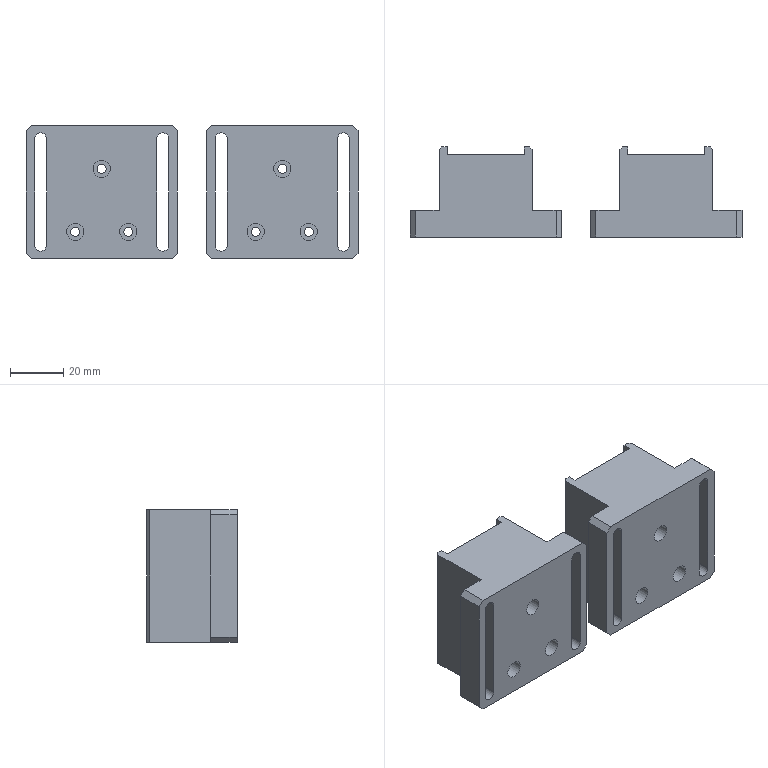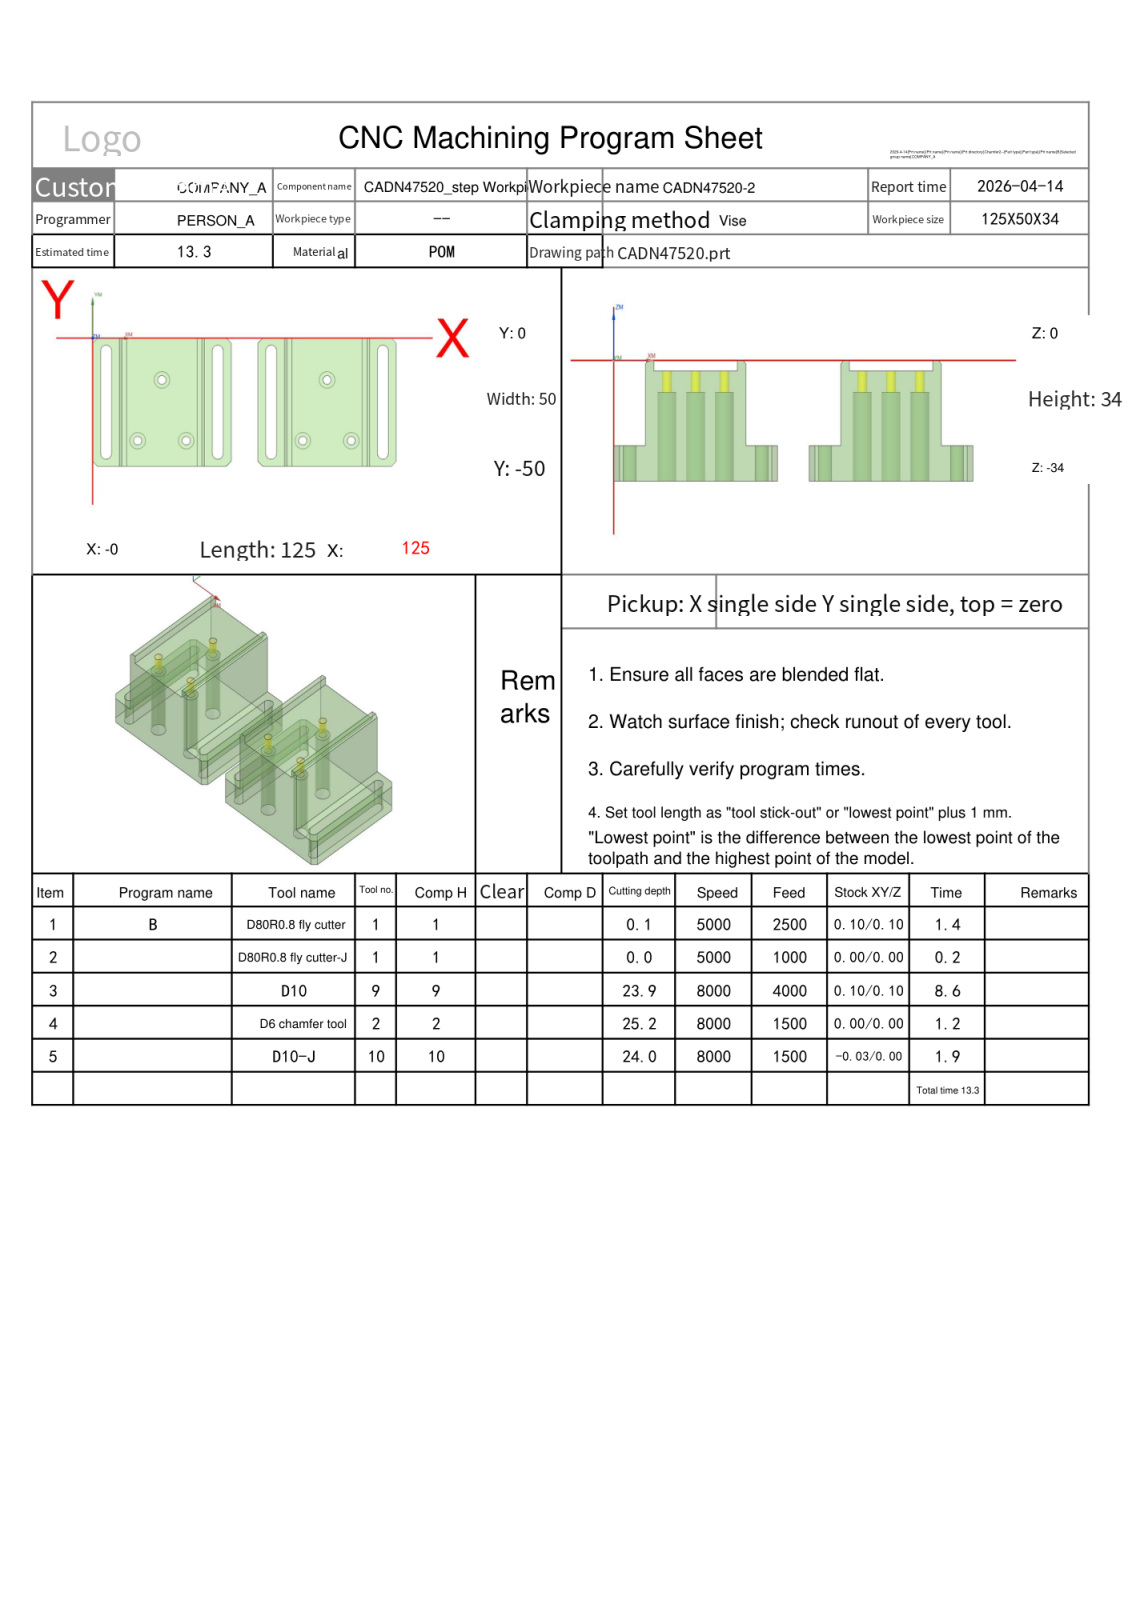NC program | NX | posted by the shop | part box 125 x 34 x 50 mm
Lines 1 to 132 of 4293:
%
O0001
(Machine time: 14.15 MIN)
(===Total Tool:4===)
(T1=D80R0.8 fly cutter D=80.  R=0.8  D-  H01 Z=0.    )
(T9=D10     D=10.  R=0.   D-  H09 Z=-23.9 )
(T2=D6 chamfer tool   D=6.   R=0.   D-  H02 Z=-25.2 )
(T10=D10-J  D=10.  R=0.   D10 H10 Z=-24.  )
G80 G90 G17 G49 G40
G91 G28 Z0
M01
N1 T01 M06
(D80R0.8 fly cutter  D=80. R=0.8 H=01 ce=0.10 di=0.10)
G00 G90 G54 X-52.097 Y-23.903 M03 S5000
G43 H01 Z20.
M08
Z7.508
G01 Z5.508 F2500.
X-40.097
X165.097
X177.097
Z7.508
G00 X-52.097
Z7.017
G01 Z5.017
X-40.097
X165.097
X177.097
Z7.017
G00 X-52.097
Z6.525
G01 Z4.525
X-40.097
X165.097
X177.097
Z6.525
G00 X-52.097
Z6.033
G01 Z4.033
X-40.097
X165.097
X177.097
Z6.033
G00 Z20.
X-52.097
Z5.542
G01 Z3.542
X-40.097
X165.097
X177.097
Z5.542
G00 Z20.
X-52.097
Z5.05
G01 Z3.05
X-40.097
X165.097
X177.097
Z5.05
G00 Z20.
X-52.097
Z4.558
G01 Z2.558
X-40.097
X165.097
X177.097
Z4.558
G00 Z20.
X-52.097
Z4.067
G01 Z2.067
X-40.097
X165.097
X177.097
Z4.067
G00 Z20.
X-52.097
Z3.575
G01 Z1.575
X-40.097
X165.097
X177.097
Z3.575
G00 Z20.
X-52.097
Z3.083
G01 Z1.083
X-40.097
X165.097
X177.097
Z3.083
G00 Z20.
X-52.097
Z2.592
G01 Z.592
X-40.097
X165.097
X177.097
Z2.592
G00 Z20.
X-52.097
Z2.1
G01 Z.1
X-40.097
X165.097
X177.097
Z2.1
G00 Z20.
G91 G28 Z0.0
M05
M09
G91 G28 Z0.0
M01
N2 T01 M06
(D80R0.8 fly cutter-J  D=80. R=0.8 H=01 ce=0.00 di=0.00)
G00 G90 G54 X-51.999 Y-24.001 M03 S5000
G43 H01 Z20.
M08
Z2.
G01 Z0.0 F1000.
X-39.999
X164.999
X176.999
Z2.
G00 Z20.
G91 G28 Z0.0
M05
M09
G91 G28 Z0.0
M01